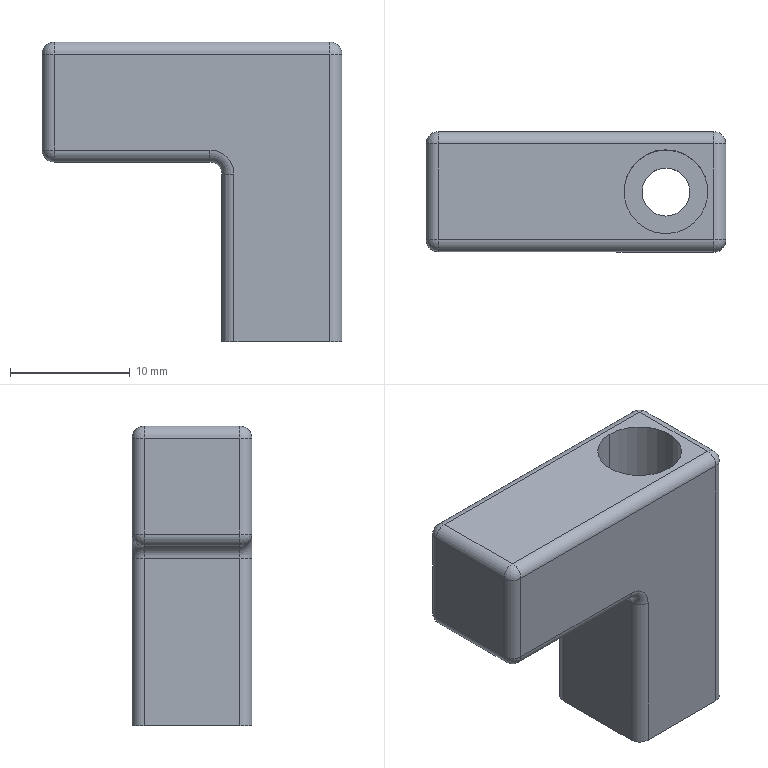NC program | NX | posted with a generic post | part box 25 x 10 x 25 mm
Whole program:
N10 G17 G21 G94 G90
(FLOOR_WALL_1 , TOOL : D10)
N12 T09 M6
N14 G54
N16 G17 G0 G90 X19. Y4.33 S9500 M3
N18 G43 Z30. H9
N20 Z0.507
N22 G94 G1 Z-0.993 F1000.
N24 X13. Y0.866
N26 G3 X12.5 Y0. R1.
N28 G1 Y-5. F2500.
N30 X2.517
N32 G3 X2.6 Y-4. R6.1
N34 G1 Y4.
N36 G3 X2.517 Y5. R6.1
N38 G1 X12.5
N40 Y0.
N42 X8.
N44 Y-0.5
N46 X7.1
N48 Y0.5
N50 X8.
N52 Y0.
N54 G3 X8.5 Y-0.866 R1.
N56 G1 Z0.507
N58 G0 X19. Y4.33 Z-0.487
N60 G1 Z-1.987 F1000.
N62 X13. Y0.866
N64 G3 X12.5 Y0. R1.
N66 G1 Y-5. F2500.
N68 X2.517
N70 G3 X2.6 Y-4. R6.1
N72 G1 Y4.
N74 G3 X2.517 Y5. R6.1
N76 G1 X12.5
N78 Y0.
N80 X8.
N82 Y-0.5
N84 X7.1
N86 Y0.5
N88 X8.
N90 Y0.
N92 G3 X8.5 Y-0.866 R1.
N94 G1 Z-0.487
N96 G0 X19. Y4.33 Z-1.48
N98 G1 Z-2.98 F1000.
N100 X13. Y0.866
N102 G3 X12.5 Y0. R1.
N104 G1 Y-5. F2500.
N106 X2.517
N108 G3 X2.6 Y-4. R6.1
N110 G1 Y4.
N112 G3 X2.517 Y5. R6.1
N114 G1 X12.5
N116 Y0.
N118 X8.
N120 Y-0.5
N122 X7.1
N124 Y0.5
N126 X8.
N128 Y0.
N130 G3 X8.5 Y-0.866 R1.
N132 G1 Z-1.48
N134 G0 X19. Y4.33 Z-2.473
N136 G1 Z-3.973 F1000.
N138 X13. Y0.866
N140 G3 X12.5 Y0. R1.
N142 G1 Y-5. F2500.
N144 X2.517
N146 G3 X2.6 Y-4. R6.1
N148 G1 Y4.
N150 G3 X2.517 Y5. R6.1
N152 G1 X12.5
N154 Y0.
N156 X8.
N158 Y-0.5
N160 X7.1
N162 Y0.5
N164 X8.
N166 Y0.
N168 G3 X8.5 Y-0.866 R1.
N170 G1 Z-2.473
N172 G0 X19. Y4.33 Z-3.467
N174 G1 Z-4.967 F1000.
N176 X13. Y0.866
N178 G3 X12.5 Y0. R1.
N180 G1 Y-5. F2500.
N182 X2.517
N184 G3 X2.6 Y-4. R6.1
N186 G1 Y4.
N188 G3 X2.517 Y5. R6.1
N190 G1 X12.5
N192 Y0.
N194 X8.
N196 Y-0.5
N198 X7.1
N200 Y0.5
N202 X8.
N204 Y0.
N206 G3 X8.5 Y-0.866 R1.
N208 G1 Z-3.467
N210 G0 X19. Y4.33 Z-4.46
N212 G1 Z-5.96 F1000.
N214 X13. Y0.866
N216 G3 X12.5 Y0. R1.
N218 G1 Y-5. F2500.
N220 X2.517
N222 G3 X2.6 Y-4. R6.1
N224 G1 Y4.
N226 G3 X2.517 Y5. R6.1
N228 G1 X12.5
N230 Y0.
N232 X8.
N234 Y-0.5
N236 X7.1
N238 Y0.5
N240 X8.
N242 Y0.
N244 G3 X8.5 Y-0.866 R1.
N246 G1 Z-4.46
N248 G0 X19. Y4.33 Z-5.453
N250 G1 Z-6.953 F1000.
N252 X13. Y0.866
N254 G3 X12.5 Y0. R1.
N256 G1 Y-5. F2500.
N258 X2.517
N260 G3 X2.6 Y-4. R6.1
N262 G1 Y4.
N264 G3 X2.517 Y5. R6.1
N266 G1 X12.5
N268 Y0.
N270 X8.
N272 Y-0.5
N274 X7.1
N276 Y0.5
N278 X8.
N280 Y0.
N282 G3 X8.5 Y-0.866 R1.
N284 G1 Z-5.453
N286 G0 X19. Y4.33 Z-6.447
N288 G1 Z-7.947 F1000.
N290 X13. Y0.866
N292 G3 X12.5 Y0. R1.
N294 G1 Y-5. F2500.
N296 X2.517
N298 G3 X2.6 Y-4. R6.1
N300 G1 Y4.
N302 G3 X2.517 Y5. R6.1
N304 G1 X12.5
N306 Y0.
N308 X8.
N310 Y-0.5
N312 X7.1
N314 Y0.5
N316 X8.
N318 Y0.
N320 G3 X8.5 Y-0.866 R1.
N322 G1 Z-6.447
N324 G0 X19. Y4.33 Z-7.44
N326 G1 Z-8.94 F1000.
N328 X13. Y0.866
N330 G3 X12.5 Y0. R1.
N332 G1 Y-5. F2500.
N334 X2.517
N336 G3 X2.6 Y-4. R6.1
N338 G1 Y4.
N340 G3 X2.517 Y5. R6.1
N342 G1 X12.5
N344 Y0.
N346 X8.
N348 Y-0.5
N350 X7.1
N352 Y0.5
N354 X8.
N356 Y0.
N358 G3 X8.5 Y-0.866 R1.
N360 G1 Z-7.44
N362 G0 X19. Y4.33 Z-8.433
N364 G1 Z-9.933 F1000.
N366 X13. Y0.866
N368 G3 X12.5 Y0. R1.
N370 G1 Y-5. F2500.
N372 X2.517
N374 G3 X2.6 Y-4. R6.1
N376 G1 Y4.
N378 G3 X2.517 Y5. R6.1
N380 G1 X12.5
N382 Y0.
N384 X8.
N386 Y-0.5
N388 X7.1
N390 Y0.5
N392 X8.
N394 Y0.
N396 G3 X8.5 Y-0.866 R1.
N398 G1 Z-8.433
N400 G0 X19. Y4.33 Z-9.427
N402 G1 Z-10.927 F1000.
N404 X13. Y0.866
N406 G3 X12.5 Y0. R1.
N408 G1 Y-5. F2500.
N410 X2.517
N412 G3 X2.6 Y-4. R6.1
N414 G1 Y4.
N416 G3 X2.517 Y5. R6.1
N418 G1 X12.5
N420 Y0.
N422 X8.
N424 Y-0.5
N426 X7.1
N428 Y0.5
N430 X8.
N432 Y0.
N434 G3 X8.5 Y-0.866 R1.
N436 G1 Z-9.427
N438 G0 X19. Y4.33 Z-10.42
N440 G1 Z-11.92 F1000.
N442 X13. Y0.866
N444 G3 X12.5 Y0. R1.
N446 G1 Y-5. F2500.
N448 X2.517
N450 G3 X2.6 Y-4. R6.1
N452 G1 Y4.
N454 G3 X2.517 Y5. R6.1
N456 G1 X12.5
N458 Y0.
N460 X8.
N462 Y-0.5
N464 X7.1
N466 Y0.5
N468 X8.
N470 Y0.
N472 G3 X8.5 Y-0.866 R1.
N474 G1 Z-10.42
N476 G0 X19. Y4.33 Z-11.413
N478 G1 Z-12.913 F1000.
N480 X13. Y0.866
N482 G3 X12.5 Y0. R1.
N484 G1 Y-5. F2500.
N486 X2.517
N488 G3 X2.6 Y-4. R6.1
N490 G1 Y4.
N492 G3 X2.517 Y5. R6.1
N494 G1 X12.5
N496 Y0.
N498 X8.
N500 Y-0.5
N502 X7.1
N504 Y0.5
N506 X8.
N508 Y0.
N510 G3 X8.5 Y-0.866 R1.
N512 G1 Z-11.413
N514 G0 X19. Y4.33 Z-12.407
N516 G1 Z-13.907 F1000.
N518 X13. Y0.866
N520 G3 X12.5 Y0. R1.
N522 G1 Y-5. F2500.
N524 X2.517
N526 G3 X2.6 Y-4. R6.1
N528 G1 Y4.
N530 G3 X2.517 Y5. R6.1
N532 G1 X12.5
N534 Y0.
N536 X8.
N538 Y-0.5
N540 X7.1
N542 Y0.5
N544 X8.
N546 Y0.
N548 G3 X8.5 Y-0.866 R1.
N550 G1 Z-12.407
N552 G0 X19. Y4.33 Z-13.4
N554 G1 Z-14.9 F1000.
N556 X13. Y0.866
N558 G3 X12.5 Y0. R1.
N560 G1 Y-5. F2500.
N562 X3.106
N564 X3.164 Y-4.825
N566 Y-3.725
N568 X3.265
N570 G3 X3.865 Y-3.125 R0.6
N572 G1 Y3.438
N574 G3 X3.265 Y4.038 R0.6
N576 G1 X3.164
N578 Y4.924
N580 X3.136 Y5.
N582 X12.5
N584 Y0.
N586 G3 X13. Y-0.866 R1.
N588 G1 X19. Y-4.33
N590 Z-13.4
N592 G0 Z30.
N594 M5
(ZLEVEL_PROFILE_COPY_COPY_COPY , TOOL : D10JING)
N596 T10 M6
N598 G54
N600 G17 G0 G90 X-4.504 Y12. S9500 M3
N602 G43 Z30. H10
N604 Z-12.5
N606 G94 G1 Z-14. F1000.
N608 X-3.821 Y10.55
N610 G3 X-3. Y9.979 R1.
N612 G2 X2.5 Y4. R6. F1200.
N614 G1 Y-4.
N616 G2 X-3.366 Y-9.999 R6.
N618 G3 X-4.221 Y-10.518 R1.
N620 G1 X-5.033 Y-12.
N622 Z-12.5
N624 G0 Z30.
N626 M5
(ZLEVEL_PROFILE_COPY_1_COPY , TOOL : D6R0.5)
N628 T08 M6
N630 G54
N632 G17 G0 G90 X-5.193 Y9.2 S9500 M3
N634 G43 Z30. H8
N636 Z-12.6
N638 G94 G1 Z-14.1 F1000.
N640 X-4.59 Y8.272
N642 G3 X-4.055 Y8. R0.6
N644 G2 X-3.018 Y7.971 R6.447 F3000.
N646 X0.5 Y4.001 R4.002
N648 G1 Y-3.998
N650 G2 X-3.485 Y-7.998 R4.
N652 G1 X-4.055 Y-8.
N654 Z-14.2
N656 X-3.485 Y-7.998
N658 G3 X0.5 Y-3.998 R4.
N660 G1 Y3.808
N662 X0.501 Y4.001
N664 G3 X-3.018 Y7.971 R4.003
N666 X-4.055 Y8. R6.491
N668 G1 Z-14.3
N670 G2 X-3.158 Y7.985 R6.536
N672 X0.501 Y3.976 R4.
N674 G1 X0.5 Y3.808
N676 Y-3.999
N678 G2 X-3.485 Y-7.998 R3.999
N680 G1 X-4.055 Y-8.
N682 Z-14.4
N684 X-3.485 Y-7.998
N686 G3 X0.5 Y-3.999 R3.999
N688 G1 Y3.808
N690 X0.501 Y3.969
N692 G3 X-3.166 Y7.986 R4.001
N694 X-4.055 Y8. R6.582
N696 G1 Z-14.5
N698 G2 X-3.171 Y7.986 R6.628
N700 X0.501 Y3.963 R4.001
N702 G1 X0.5 Y3.808
N704 Y-4.
N706 G2 X-3.485 Y-7.998 R3.999
N708 G1 X-4.055 Y-8.
N710 Z-14.599
N712 X-3.46 Y-7.998
N714 G3 X-1.636 Y-7.538 R3.891
N716 X0.51 Y-3.989 R3.984
N718 G1 Y4.
N720 G3 X0.146 Y5.666 R3.958
N722 X-3.178 Y7.987 R4.016
N724 X-4.055 Y8. R6.675
N726 G1 Z-14.694
N728 G2 X-3.157 Y7.986 R6.72
N730 X0.092 Y5.818 R4.033
N732 G1 X0.167 Y5.661
N734 G2 X0.539 Y4.017 R3.812
N736 G1 Y-4.
N738 G2 X-1.636 Y-7.544 R4.005
N740 X-3.461 Y-7.998 R3.948
N742 G1 X-4.055 Y-8.
N744 Z-14.771
N746 X-3.364 Y-7.998
N748 G3 X0.092 Y-5.87 R4.073
N750 X0.58 Y-4. R3.854
N752 G1 Y4.
N754 G3 X0.485 Y4.846 R4.232
N756 X-3.187 Y7.988 R4.088
N758 X-4.055 Y8. R6.999
N760 G1 Z-14.847
N762 G2 X-2.673 Y7.926 R6.364
N764 X0.487 Y5.053 R4.203
N766 X0.64 Y4. R3.529
N768 G1 Y-3.988
N770 G2 X-0.368 Y-6.577 R3.906
N772 X-3.364 Y-7.998 R4.098
N774 G1 X-4.055 Y-8.
N776 Z-14.909
N778 X-3.709 Y-7.999
N780 X-3.364 Y-7.998
N782 X-3.018 Y-7.978
N784 X-2.673 Y-7.929
N786 G3 X-0.599 Y-6.854 R4.327
N788 G1 X-0.333 Y-6.577
N790 G3 X0.712 Y-3.988 R3.963
N792 G1 Y4.
N794 G3 X0.536 Y5.091 R3.431
N796 X-2.673 Y7.929 R4.315
N798 X-4.055 Y8. R6.595
N800 G1 Z-14.95
N802 G2 X-2.673 Y7.932 R6.878
N804 X0.601 Y5.067 R4.43
N806 G1 X0.64 Y4.943
N808 X0.655 Y4.886
N810 X0.67 Y4.829
N812 X0.783 Y4.137
N814 X0.782 Y4.
N816 Y-4.
N818 G2 X0.602 Y-5.064 R3.396
N820 X-1.716 Y-7.616 R4.441
N822 G1 X-1.877 Y-7.685
N824 G2 X-3.387 Y-7.998 R3.851
N826 G1 X-4.055 Y-8.
N828 Z-14.967
N830 X-3.364 Y-7.998
N832 G3 X-1.982 Y-7.732 R3.924
N834 X0.554 Y-5.271 R4.558
N836 G1 X0.614 Y-5.116
N838 G3 X0.821 Y-3.999 R3.262
N840 G1 Y4.
N842 G3 X0.635 Y5.06 R3.1
N844 G1 X0.553 Y5.273
N846 G3 X-2.673 Y7.933 R4.514
N848 X-4.055 Y8. R6.971
N850 G1 Z-14.986
N852 G2 X-2.673 Y7.934 R7.073
N854 X0.092 Y6.124 R4.501
N856 G1 X0.259 Y5.885
N858 G2 X0.881 Y4. R3.516
N860 G1 Y-4.
N862 G2 X0.259 Y-5.885 R3.522
N864 G1 X0.092 Y-6.124
N866 G2 X-2.327 Y-7.851 R4.536
N868 X-3.364 Y-7.998 R3.954
N870 G1 X-4.055 Y-8.
N872 Z-15.
N874 X-3.364 Y-7.998
N876 G3 X-2.673 Y-7.935 R5.002
N878 X-0.27 Y-6.577 R4.477
N880 X0.465 Y-5.577 R5.955
N882 X0.672 Y-5.145 R7.853
N884 G1 X0.758 Y-4.946
N886 G3 X0.95 Y-4. R2.64
N888 G1 Y3.808
N890 X0.972 Y4.022
N892 X0.946 Y4.056
N894 G3 X0.739 Y4.996 R2.71
N896 G1 X0.669 Y5.147
N898 G3 X0.463 Y5.578 R1.902
N900 X0.019 Y6.231 R4.94
N902 X-2.673 Y7.935 R4.489
N904 X-4.055 Y8. R7.146
N906 G2 X-4.589 Y8.274 R0.6
N908 G1 X-5.187 Y9.2
N910 Z-13.5
N912 G0 Z30.
(ZLEVEL_PROFILE_COPY_1_COPY_COPY , TOOL : D6R0.5)
N914 X-0.256 Y8.172
N916 Z-13.512
N918 G1 Z-15.012 F1000.
N920 X-0.514 Y7.273
N922 G3 X-0.369 Y6.69 R0.6
N924 G1 X11.5 F3000.
N926 G2 X14.19 Y4. R2.69
N928 G1 Y-4.
N930 G2 X11.5 Y-6.69 R2.69
N932 G1 X-0.369
N934 X-0.463 Y-6.8 Z-15.03
N936 X11.5
N938 G3 X14.3 Y-4. R2.8
N940 G1 Y4.
N942 G3 X11.5 Y6.8 R2.8
N944 G1 X-0.463
N946 X-0.563 Y6.903 Z-15.055
N948 X11.5
N950 G2 X14.403 Y4. R2.903
N952 G1 Y-4.
N954 G2 X11.5 Y-6.903 R2.903
N956 G1 X-0.563
N958 X-0.656 Y-7.002 Z-15.086
N960 X11.5
N962 G3 X14.502 Y-4. R3.002
N964 G1 Y4.
N966 G3 X11.5 Y7.002 R3.002
N968 G1 X-0.646
N970 X-0.744 Y7.097 Z-15.124
N972 X11.5
N974 G2 X14.597 Y4. R3.097
N976 G1 Y-4.
N978 G2 X11.5 Y-7.097 R3.097
N980 G1 X-0.745
N982 X-0.841 Y-7.189 Z-15.167
N984 X11.5
N986 G3 X14.689 Y-4. R3.189
N988 G1 Y4.
N990 G3 X11.5 Y7.189 R3.189
N992 G1 X-0.839
N994 X-0.929 Y7.277 Z-15.217
N996 X11.5
N998 G2 X14.777 Y4. R3.277
N1000 G1 Y-4.
N1002 G2 X11.5 Y-7.277 R3.277
N1004 G1 X-0.943
N1006 X-1.031 Y-7.361 Z-15.272
N1008 X11.5
N1010 G3 X14.861 Y-4. R3.361
N1012 G1 Y4.
N1014 G3 X11.5 Y7.361 R3.361
N1016 G1 X-1.02
N1018 X-1.102 Y7.442 Z-15.333
N1020 X11.5
N1022 G2 X14.942 Y4. R3.442
N1024 G1 Y-4.
N1026 G2 X11.5 Y-7.442 R3.442
N1028 G1 X-1.101
N1030 X-1.179 Y-7.518 Z-15.398
N1032 X11.5
N1034 G3 X15.018 Y-4. R3.518
N1036 G1 Y4.
N1038 G3 X11.5 Y7.518 R3.518
N1040 G1 X-1.18
N1042 X-1.271 Y7.589 Z-15.469
N1044 X11.5
N1046 G2 X15.089 Y4. R3.589
N1048 G1 Y-4.
N1050 G2 X11.5 Y-7.589 R3.589
N1052 G1 X-1.271
N1054 X-1.35 Y-7.656 Z-15.544
N1056 X11.5
N1058 G3 X15.156 Y-4. R3.656
N1060 G1 Y4.
N1062 G3 X11.5 Y7.656 R3.656
N1064 G1 X-1.35
N1066 X-1.42 Y7.717 Z-15.623
N1068 X11.5
N1070 G2 X15.217 Y4. R3.717
N1072 G1 Y-4.
N1074 G2 X11.5 Y-7.717 R3.717
N1076 G1 X-1.42
N1078 X-1.5 Y-7.773 Z-15.707
N1080 X11.5
N1082 G3 X15.273 Y-4. R3.773
N1084 G1 Y4.
N1086 G3 X11.5 Y7.773 R3.773
N1088 G1 X-1.5
N1090 X-1.624 Y7.805
N1092 X-1.71 Y7.855 Z-15.793
N1094 X-1.593 Y7.835
N1096 X-1.544 Y7.826
N1098 X-1.5 Y7.823
N1100 X11.5
N1102 G2 X15.323 Y4. R3.823
N1104 G1 Y-4.
N1106 G2 X11.5 Y-7.823 R3.823
N1108 G1 X-1.5
N1110 X-1.674 Y-7.849
N1112 X-1.792 Y-7.895 Z-15.883
N1114 X-1.5 Y-7.867
N1116 X11.5
N1118 G3 X15.367 Y-4. R3.867
N1120 G1 Y4.
N1122 G3 X11.5 Y7.867 R3.867
N1124 G1 X-1.5
N1126 X-1.544
N1128 X-1.791 Y7.895
N1130 X-1.882 Y7.932 Z-15.976
N1132 G3 X-1.5 Y7.905 R2.935
N1134 G1 X11.5
N1136 G2 X15.405 Y4. R3.905
N1138 G1 Y-4.
N1140 G2 X11.5 Y-7.905 R3.905
N1142 G1 X-1.5
N1144 G3 X-1.882 Y-7.932 R3.263
N1146 G1 X-2.01 Y-7.965 Z-16.071
N1148 G2 X-1.5 Y-7.937 R4.227
N1150 G1 X11.5
N1152 G3 X15.437 Y-4. R3.937
N1154 G1 Y4.
N1156 G3 X11.5 Y7.937 R3.937
N1158 G1 X-1.5
N1160 X-1.543 Y7.933
N1162 X-2.01 Y7.965
N1164 X-1.904 Y7.972 Z-16.168
N1166 X-1.5 Y7.963
N1168 X11.5
N1170 G2 X15.463 Y4. R3.963
N1172 G1 Y-4.
N1174 G2 X11.5 Y-7.963 R3.963
N1176 G1 X-1.5
N1178 X-1.904 Y-7.972
N1180 Y-7.982 Z-16.251
N1182 X-1.5 Y-7.979
N1184 X11.5
N1186 G3 X15.479 Y-4. R3.979
N1188 G1 Y4.
N1190 G3 X11.5 Y7.979 R3.979
N1192 G1 X-1.5
N1194 X-1.904 Y7.982
N1196 Y7.992 Z-16.334
N1198 X-1.5 Y7.991
N1200 X11.5
N1202 G2 X15.491 Y4. R3.991
N1204 G1 Y-4.
N1206 G2 X11.5 Y-7.991 R3.991
N1208 G1 X-1.5
N1210 X-1.904 Y-7.992
N1212 X-2.076 Y-8. Z-16.417
N1214 X-1.5 Y-7.998
N1216 X11.5
N1218 G3 X15.498 Y-4. R3.998
N1220 G1 Y4.
N1222 G3 X11.5 Y7.998 R3.998
N1224 G1 X-1.5
N1226 X-2.076 Y8.
N1228 Z-16.5
N1230 X11.5
N1232 G2 X15.5 Y4. R4.002
N1234 G1 Y-3.808
N1236 X15.498 Y-4.
N1238 G2 X13.752 Y-7.303 R3.99
N1240 X13.135 Y-7.648 R3.57
N1242 X12.06 Y-7.958 R4.059
N1244 X11.496 Y-7.999 R3.967
N1246 G1 X-1.732 Y-7.997
N1248 X-2.076 Y-8.
N1250 G3 X-2.593 Y-8.304 R0.6
N1252 G1 X-3.101 Y-9.2
N1254 Z-15.
N1256 G0 Z30.
N1258 M5
N1260 M2